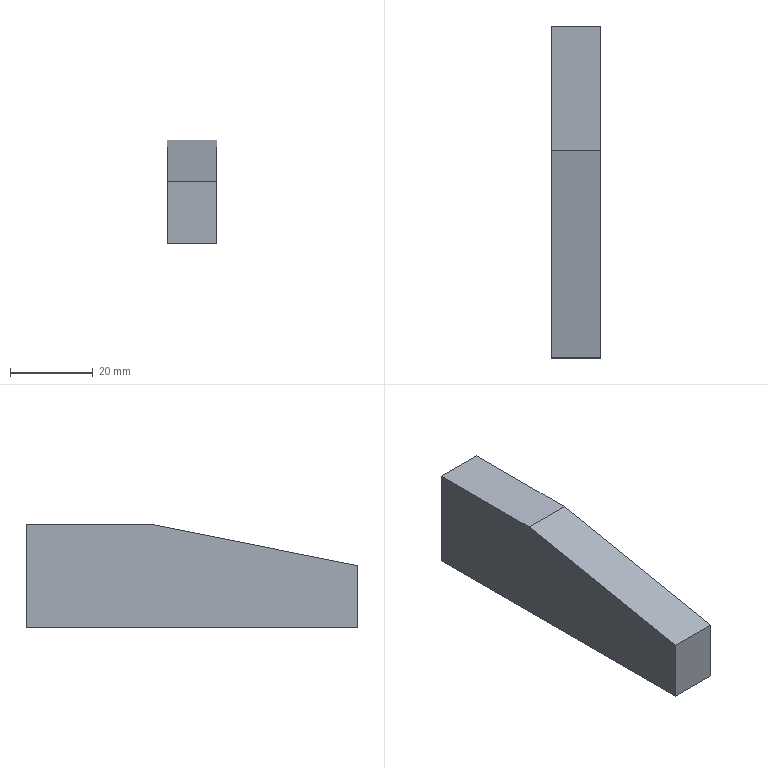Part | NX | 1 solid | 15 faces | box 12 x 80 x 25 mm | volume 20028 mm3 | plane 7 | cone 4 | cylinder 4 | commonest cylinder face diameters 5 x3 3 x1
STEP:
#1=CARTESIAN_POINT('',(0.,19.5,-12.5));
#2=VERTEX_POINT('',#1);
#3=CARTESIAN_POINT('',(0.,17.,-12.5));
#4=DIRECTION('',(0.,0.,-1.));
#5=DIRECTION('',(0.,1.,0.));
#6=AXIS2_PLACEMENT_3D('',#3,#4,#5);
#7=CIRCLE('',#6,2.5);
#8=EDGE_CURVE('',#2,#2,#7,.T.);
#9=ORIENTED_EDGE('',*,*,#8,.F.);
#10=EDGE_LOOP('',(#9));
#11=FACE_BOUND('',#10,.T.);
#12=CARTESIAN_POINT('',(0.,-25.5,-12.5));
#13=VERTEX_POINT('',#12);
#14=CARTESIAN_POINT('',(0.,-28.,-12.5));
#15=DIRECTION('',(0.,0.,-1.));
#16=DIRECTION('',(0.,1.,0.));
#17=AXIS2_PLACEMENT_3D('',#14,#15,#16);
#18=CIRCLE('',#17,2.5);
#19=EDGE_CURVE('',#13,#13,#18,.T.);
#20=ORIENTED_EDGE('',*,*,#19,.F.);
#21=EDGE_LOOP('',(#20));
#22=FACE_BOUND('',#21,.T.);
#23=CARTESIAN_POINT('',(-6.,-40.,-12.5));
#24=VERTEX_POINT('',#23);
#25=CARTESIAN_POINT('',(-6.,40.,-12.5));
#26=VERTEX_POINT('',#25);
#27=CARTESIAN_POINT('',(-6.,40.,-12.5));
#28=DIRECTION('',(0.,1.,0.));
#29=VECTOR('',#28,1000.);
#30=LINE('',#27,#29);
#31=EDGE_CURVE('',#24,#26,#30,.T.);
#32=ORIENTED_EDGE('',*,*,#31,.T.);
#33=CARTESIAN_POINT('',(6.,40.,-12.5));
#34=VERTEX_POINT('',#33);
#35=CARTESIAN_POINT('',(6.,40.,-12.5));
#36=DIRECTION('',(-1.,0.,0.));
#37=VECTOR('',#36,1000.);
#38=LINE('',#35,#37);
#39=EDGE_CURVE('',#34,#26,#38,.T.);
#40=ORIENTED_EDGE('',*,*,#39,.F.);
#41=CARTESIAN_POINT('',(6.,-40.,-12.5));
#42=VERTEX_POINT('',#41);
#43=CARTESIAN_POINT('',(6.,40.,-12.5));
#44=DIRECTION('',(0.,1.,0.));
#45=VECTOR('',#44,1000.);
#46=LINE('',#43,#45);
#47=EDGE_CURVE('',#42,#34,#46,.T.);
#48=ORIENTED_EDGE('',*,*,#47,.F.);
#49=CARTESIAN_POINT('',(6.,-40.,-12.5));
#50=DIRECTION('',(-1.,0.,0.));
#51=VECTOR('',#50,1000.);
#52=LINE('',#49,#51);
#53=EDGE_CURVE('',#42,#24,#52,.T.);
#54=ORIENTED_EDGE('',*,*,#53,.T.);
#55=EDGE_LOOP('',(#32,#40,#48,#54));
#56=FACE_BOUND('',#55,.T.);
#57=CARTESIAN_POINT('',(6.,40.,-12.5));
#58=DIRECTION('',(0.,0.,1.));
#59=DIRECTION('',(0.,-1.,0.));
#60=AXIS2_PLACEMENT_3D('',#57,#58,#59);
#61=PLANE('',#60);
#62=ADVANCED_FACE('',(#11,#22,#56),#61,.F.);
#63=CARTESIAN_POINT('',(0.,40.,9.));
#64=VERTEX_POINT('',#63);
#65=CARTESIAN_POINT('',(0.,40.,7.5));
#66=DIRECTION('',(0.,1.,0.));
#67=DIRECTION('',(0.,0.,1.));
#68=AXIS2_PLACEMENT_3D('',#65,#66,#67);
#69=CIRCLE('',#68,1.5);
#70=EDGE_CURVE('',#64,#64,#69,.T.);
#71=ORIENTED_EDGE('',*,*,#70,.F.);
#72=EDGE_LOOP('',(#71));
#73=FACE_BOUND('',#72,.T.);
#74=CARTESIAN_POINT('',(0.,40.,0.));
#75=VERTEX_POINT('',#74);
#76=CARTESIAN_POINT('',(0.,40.,-2.5));
#77=DIRECTION('',(0.,1.,0.));
#78=DIRECTION('',(0.,0.,1.));
#79=AXIS2_PLACEMENT_3D('',#76,#77,#78);
#80=CIRCLE('',#79,2.5);
#81=EDGE_CURVE('',#75,#75,#80,.T.);
#82=ORIENTED_EDGE('',*,*,#81,.F.);
#83=EDGE_LOOP('',(#82));
#84=FACE_BOUND('',#83,.T.);
#85=CARTESIAN_POINT('',(-6.,40.,12.5));
#86=VERTEX_POINT('',#85);
#87=CARTESIAN_POINT('',(-6.,40.,12.5));
#88=DIRECTION('',(0.,0.,1.));
#89=VECTOR('',#88,1000.);
#90=LINE('',#87,#89);
#91=EDGE_CURVE('',#26,#86,#90,.T.);
#92=ORIENTED_EDGE('',*,*,#91,.T.);
#93=CARTESIAN_POINT('',(6.,40.,12.5));
#94=VERTEX_POINT('',#93);
#95=CARTESIAN_POINT('',(6.,40.,12.5));
#96=DIRECTION('',(-1.,0.,0.));
#97=VECTOR('',#96,1000.);
#98=LINE('',#95,#97);
#99=EDGE_CURVE('',#94,#86,#98,.T.);
#100=ORIENTED_EDGE('',*,*,#99,.F.);
#101=CARTESIAN_POINT('',(6.,40.,12.5));
#102=DIRECTION('',(0.,0.,1.));
#103=VECTOR('',#102,1000.);
#104=LINE('',#101,#103);
#105=EDGE_CURVE('',#34,#94,#104,.T.);
#106=ORIENTED_EDGE('',*,*,#105,.F.);
#107=ORIENTED_EDGE('',*,*,#39,.T.);
#108=EDGE_LOOP('',(#92,#100,#106,#107));
#109=FACE_BOUND('',#108,.T.);
#110=CARTESIAN_POINT('',(6.,40.,12.5));
#111=DIRECTION('',(0.,-1.,0.));
#112=DIRECTION('',(0.,0.,-1.));
#113=AXIS2_PLACEMENT_3D('',#110,#111,#112);
#114=PLANE('',#113);
#115=ADVANCED_FACE('',(#73,#84,#109),#114,.F.);
#116=CARTESIAN_POINT('',(-6.,10.,12.5));
#117=VERTEX_POINT('',#116);
#118=CARTESIAN_POINT('',(-6.,40.,12.5));
#119=DIRECTION('',(0.,-1.,0.));
#120=VECTOR('',#119,1000.);
#121=LINE('',#118,#120);
#122=EDGE_CURVE('',#86,#117,#121,.T.);
#123=ORIENTED_EDGE('',*,*,#122,.T.);
#124=CARTESIAN_POINT('',(6.,10.,12.5));
#125=VERTEX_POINT('',#124);
#126=CARTESIAN_POINT('',(6.,10.,12.5));
#127=DIRECTION('',(1.,0.,0.));
#128=VECTOR('',#127,1000.);
#129=LINE('',#126,#128);
#130=EDGE_CURVE('',#117,#125,#129,.T.);
#131=ORIENTED_EDGE('',*,*,#130,.T.);
#132=CARTESIAN_POINT('',(6.,40.,12.5));
#133=DIRECTION('',(0.,-1.,0.));
#134=VECTOR('',#133,1000.);
#135=LINE('',#132,#134);
#136=EDGE_CURVE('',#94,#125,#135,.T.);
#137=ORIENTED_EDGE('',*,*,#136,.F.);
#138=ORIENTED_EDGE('',*,*,#99,.T.);
#139=EDGE_LOOP('',(#123,#131,#137,#138));
#140=FACE_BOUND('',#139,.T.);
#141=CARTESIAN_POINT('',(6.,40.,12.5));
#142=DIRECTION('',(0.,0.,-1.));
#143=DIRECTION('',(0.,1.,0.));
#144=AXIS2_PLACEMENT_3D('',#141,#142,#143);
#145=PLANE('',#144);
#146=ADVANCED_FACE('',(#140),#145,.F.);
#147=CARTESIAN_POINT('',(6.,-40.,2.5));
#148=VERTEX_POINT('',#147);
#149=CARTESIAN_POINT('',(6.,-40.,12.5));
#150=DIRECTION('',(0.,0.,-1.));
#151=VECTOR('',#150,1000.);
#152=LINE('',#149,#151);
#153=EDGE_CURVE('',#148,#42,#152,.T.);
#154=ORIENTED_EDGE('',*,*,#153,.F.);
#155=CARTESIAN_POINT('',(-6.,-40.,2.5));
#156=VERTEX_POINT('',#155);
#157=CARTESIAN_POINT('',(6.,-40.,2.5));
#158=DIRECTION('',(-1.,0.,0.));
#159=VECTOR('',#158,1000.);
#160=LINE('',#157,#159);
#161=EDGE_CURVE('',#148,#156,#160,.T.);
#162=ORIENTED_EDGE('',*,*,#161,.T.);
#163=CARTESIAN_POINT('',(-6.,-40.,12.5));
#164=DIRECTION('',(0.,0.,-1.));
#165=VECTOR('',#164,1000.);
#166=LINE('',#163,#165);
#167=EDGE_CURVE('',#156,#24,#166,.T.);
#168=ORIENTED_EDGE('',*,*,#167,.T.);
#169=ORIENTED_EDGE('',*,*,#53,.F.);
#170=EDGE_LOOP('',(#154,#162,#168,#169));
#171=FACE_BOUND('',#170,.T.);
#172=CARTESIAN_POINT('',(6.,-40.,12.5));
#173=DIRECTION('',(0.,1.,0.));
#174=DIRECTION('',(0.,0.,1.));
#175=AXIS2_PLACEMENT_3D('',#172,#173,#174);
#176=PLANE('',#175);
#177=ADVANCED_FACE('',(#171),#176,.F.);
#178=ORIENTED_EDGE('',*,*,#136,.T.);
#179=CARTESIAN_POINT('',(6.,-2.019,10.096));
#180=DIRECTION('',(0.,0.9806,0.1961));
#181=VECTOR('',#180,1000.);
#182=LINE('',#179,#181);
#183=EDGE_CURVE('',#125,#148,#182,.F.);
#184=ORIENTED_EDGE('',*,*,#183,.T.);
#185=ORIENTED_EDGE('',*,*,#153,.T.);
#186=ORIENTED_EDGE('',*,*,#47,.T.);
#187=ORIENTED_EDGE('',*,*,#105,.T.);
#188=EDGE_LOOP('',(#178,#184,#185,#186,#187));
#189=FACE_BOUND('',#188,.T.);
#190=CARTESIAN_POINT('',(6.,0.,0.));
#191=DIRECTION('',(1.,0.,0.));
#192=DIRECTION('',(0.,0.,-1.));
#193=AXIS2_PLACEMENT_3D('',#190,#191,#192);
#194=PLANE('',#193);
#195=ADVANCED_FACE('',(#189),#194,.T.);
#196=ORIENTED_EDGE('',*,*,#167,.F.);
#197=CARTESIAN_POINT('',(-6.,-40.,2.5));
#198=DIRECTION('',(0.,-0.9806,-0.1961));
#199=VECTOR('',#198,1000.);
#200=LINE('',#197,#199);
#201=EDGE_CURVE('',#156,#117,#200,.F.);
#202=ORIENTED_EDGE('',*,*,#201,.T.);
#203=ORIENTED_EDGE('',*,*,#122,.F.);
#204=ORIENTED_EDGE('',*,*,#91,.F.);
#205=ORIENTED_EDGE('',*,*,#31,.F.);
#206=EDGE_LOOP('',(#196,#202,#203,#204,#205));
#207=FACE_BOUND('',#206,.T.);
#208=CARTESIAN_POINT('',(-6.,0.,0.));
#209=DIRECTION('',(1.,0.,0.));
#210=DIRECTION('',(0.,0.,-1.));
#211=AXIS2_PLACEMENT_3D('',#208,#209,#210);
#212=PLANE('',#211);
#213=ADVANCED_FACE('',(#207),#212,.F.);
#214=CARTESIAN_POINT('',(0.,-28.,4.002));
#215=VERTEX_POINT('',#214);
#216=VERTEX_LOOP('',#215);
#217=FACE_BOUND('',#216,.T.);
#218=CARTESIAN_POINT('',(0.,-25.5,2.5));
#219=VERTEX_POINT('',#218);
#220=CARTESIAN_POINT('',(0.,-28.,2.5));
#221=DIRECTION('',(0.,0.,-1.));
#222=DIRECTION('',(0.,1.,0.));
#223=AXIS2_PLACEMENT_3D('',#220,#221,#222);
#224=CIRCLE('',#223,2.5);
#225=EDGE_CURVE('',#219,#219,#224,.T.);
#226=ORIENTED_EDGE('',*,*,#225,.T.);
#227=EDGE_LOOP('',(#226));
#228=FACE_BOUND('',#227,.T.);
#229=CARTESIAN_POINT('',(0.,-28.,2.5));
#230=DIRECTION('',(0.,0.,-1.));
#231=DIRECTION('',(0.,1.,0.));
#232=AXIS2_PLACEMENT_3D('',#229,#230,#231);
#233=CONICAL_SURFACE('',#232,2.5,1.03);
#234=ADVANCED_FACE('',(#217,#228),#233,.F.);
#235=ORIENTED_EDGE('',*,*,#225,.F.);
#236=EDGE_LOOP('',(#235));
#237=FACE_BOUND('',#236,.T.);
#238=ORIENTED_EDGE('',*,*,#19,.T.);
#239=EDGE_LOOP('',(#238));
#240=FACE_BOUND('',#239,.T.);
#241=CARTESIAN_POINT('',(0.,-28.,-12.5));
#242=DIRECTION('',(0.,0.,-1.));
#243=DIRECTION('',(0.,1.,0.));
#244=AXIS2_PLACEMENT_3D('',#241,#242,#243);
#245=CYLINDRICAL_SURFACE('',#244,2.5);
#246=ADVANCED_FACE('',(#237,#240),#245,.F.);
#247=CARTESIAN_POINT('',(0.,17.,4.002));
#248=VERTEX_POINT('',#247);
#249=VERTEX_LOOP('',#248);
#250=FACE_BOUND('',#249,.T.);
#251=CARTESIAN_POINT('',(0.,19.5,2.5));
#252=VERTEX_POINT('',#251);
#253=CARTESIAN_POINT('',(0.,17.,2.5));
#254=DIRECTION('',(0.,0.,-1.));
#255=DIRECTION('',(0.,1.,0.));
#256=AXIS2_PLACEMENT_3D('',#253,#254,#255);
#257=CIRCLE('',#256,2.5);
#258=EDGE_CURVE('',#252,#252,#257,.T.);
#259=ORIENTED_EDGE('',*,*,#258,.T.);
#260=EDGE_LOOP('',(#259));
#261=FACE_BOUND('',#260,.T.);
#262=CARTESIAN_POINT('',(0.,17.,2.5));
#263=DIRECTION('',(0.,0.,-1.));
#264=DIRECTION('',(0.,1.,0.));
#265=AXIS2_PLACEMENT_3D('',#262,#263,#264);
#266=CONICAL_SURFACE('',#265,2.5,1.03);
#267=ADVANCED_FACE('',(#250,#261),#266,.F.);
#268=ORIENTED_EDGE('',*,*,#258,.F.);
#269=EDGE_LOOP('',(#268));
#270=FACE_BOUND('',#269,.T.);
#271=ORIENTED_EDGE('',*,*,#8,.T.);
#272=EDGE_LOOP('',(#271));
#273=FACE_BOUND('',#272,.T.);
#274=CARTESIAN_POINT('',(0.,17.,-12.5));
#275=DIRECTION('',(0.,0.,-1.));
#276=DIRECTION('',(0.,1.,0.));
#277=AXIS2_PLACEMENT_3D('',#274,#275,#276);
#278=CYLINDRICAL_SURFACE('',#277,2.5);
#279=ADVANCED_FACE('',(#270,#273),#278,.F.);
#280=CARTESIAN_POINT('',(0.,23.498,-2.5));
#281=VERTEX_POINT('',#280);
#282=VERTEX_LOOP('',#281);
#283=FACE_BOUND('',#282,.T.);
#284=CARTESIAN_POINT('',(0.,25.,0.));
#285=VERTEX_POINT('',#284);
#286=CARTESIAN_POINT('',(0.,25.,-2.5));
#287=DIRECTION('',(0.,1.,0.));
#288=DIRECTION('',(0.,0.,1.));
#289=AXIS2_PLACEMENT_3D('',#286,#287,#288);
#290=CIRCLE('',#289,2.5);
#291=EDGE_CURVE('',#285,#285,#290,.T.);
#292=ORIENTED_EDGE('',*,*,#291,.T.);
#293=EDGE_LOOP('',(#292));
#294=FACE_BOUND('',#293,.T.);
#295=CARTESIAN_POINT('',(0.,25.,-2.5));
#296=DIRECTION('',(0.,1.,0.));
#297=DIRECTION('',(0.,0.,1.));
#298=AXIS2_PLACEMENT_3D('',#295,#296,#297);
#299=CONICAL_SURFACE('',#298,2.5,1.03);
#300=ADVANCED_FACE('',(#283,#294),#299,.F.);
#301=ORIENTED_EDGE('',*,*,#291,.F.);
#302=EDGE_LOOP('',(#301));
#303=FACE_BOUND('',#302,.T.);
#304=ORIENTED_EDGE('',*,*,#81,.T.);
#305=EDGE_LOOP('',(#304));
#306=FACE_BOUND('',#305,.T.);
#307=CARTESIAN_POINT('',(0.,40.,-2.5));
#308=DIRECTION('',(0.,1.,0.));
#309=DIRECTION('',(0.,0.,1.));
#310=AXIS2_PLACEMENT_3D('',#307,#308,#309);
#311=CYLINDRICAL_SURFACE('',#310,2.5);
#312=ADVANCED_FACE('',(#303,#306),#311,.F.);
#313=ORIENTED_EDGE('',*,*,#183,.F.);
#314=ORIENTED_EDGE('',*,*,#130,.F.);
#315=ORIENTED_EDGE('',*,*,#201,.F.);
#316=ORIENTED_EDGE('',*,*,#161,.F.);
#317=EDGE_LOOP('',(#313,#314,#315,#316));
#318=FACE_BOUND('',#317,.T.);
#319=CARTESIAN_POINT('',(6.,-40.,2.5));
#320=DIRECTION('',(0.,0.1961,-0.9806));
#321=DIRECTION('',(-1.,0.,0.));
#322=AXIS2_PLACEMENT_3D('',#319,#320,#321);
#323=PLANE('',#322);
#324=ADVANCED_FACE('',(#318),#323,.F.);
#325=CARTESIAN_POINT('',(0.,31.099,7.5));
#326=VERTEX_POINT('',#325);
#327=VERTEX_LOOP('',#326);
#328=FACE_BOUND('',#327,.T.);
#329=CARTESIAN_POINT('',(0.,32.,9.));
#330=VERTEX_POINT('',#329);
#331=CARTESIAN_POINT('',(0.,32.,7.5));
#332=DIRECTION('',(0.,1.,0.));
#333=DIRECTION('',(0.,0.,1.));
#334=AXIS2_PLACEMENT_3D('',#331,#332,#333);
#335=CIRCLE('',#334,1.5);
#336=EDGE_CURVE('',#330,#330,#335,.T.);
#337=ORIENTED_EDGE('',*,*,#336,.T.);
#338=EDGE_LOOP('',(#337));
#339=FACE_BOUND('',#338,.T.);
#340=CARTESIAN_POINT('',(0.,32.,7.5));
#341=DIRECTION('',(0.,1.,0.));
#342=DIRECTION('',(0.,0.,1.));
#343=AXIS2_PLACEMENT_3D('',#340,#341,#342);
#344=CONICAL_SURFACE('',#343,1.5,1.03);
#345=ADVANCED_FACE('',(#328,#339),#344,.F.);
#346=ORIENTED_EDGE('',*,*,#336,.F.);
#347=EDGE_LOOP('',(#346));
#348=FACE_BOUND('',#347,.T.);
#349=ORIENTED_EDGE('',*,*,#70,.T.);
#350=EDGE_LOOP('',(#349));
#351=FACE_BOUND('',#350,.T.);
#352=CARTESIAN_POINT('',(0.,40.,7.5));
#353=DIRECTION('',(0.,1.,0.));
#354=DIRECTION('',(0.,0.,1.));
#355=AXIS2_PLACEMENT_3D('',#352,#353,#354);
#356=CYLINDRICAL_SURFACE('',#355,1.5);
#357=ADVANCED_FACE('',(#348,#351),#356,.F.);
#358=CLOSED_SHELL('',(#62,#115,#146,#177,#195,#213,#234,#246,#267,#279,#300,#312,#324,#345,#357));
#359=MANIFOLD_SOLID_BREP('',#358);
#360=(LENGTH_UNIT()NAMED_UNIT(*)SI_UNIT(.MILLI.,.METRE.));
#361=UNCERTAINTY_MEASURE_WITH_UNIT(LENGTH_MEASURE(0.00001),#360,'','');
#362=(NAMED_UNIT(*)PLANE_ANGLE_UNIT()SI_UNIT($,.RADIAN.));
#363=(NAMED_UNIT(*)SI_UNIT($,.STERADIAN.)SOLID_ANGLE_UNIT());
#364=(GEOMETRIC_REPRESENTATION_CONTEXT(3)GLOBAL_UNCERTAINTY_ASSIGNED_CONTEXT((#361))GLOBAL_UNIT_ASSIGNED_CONTEXT((#360,#362,#363))REPRESENTATION_CONTEXT('',''));
#365=ADVANCED_BREP_SHAPE_REPRESENTATION('',(#359),#364);